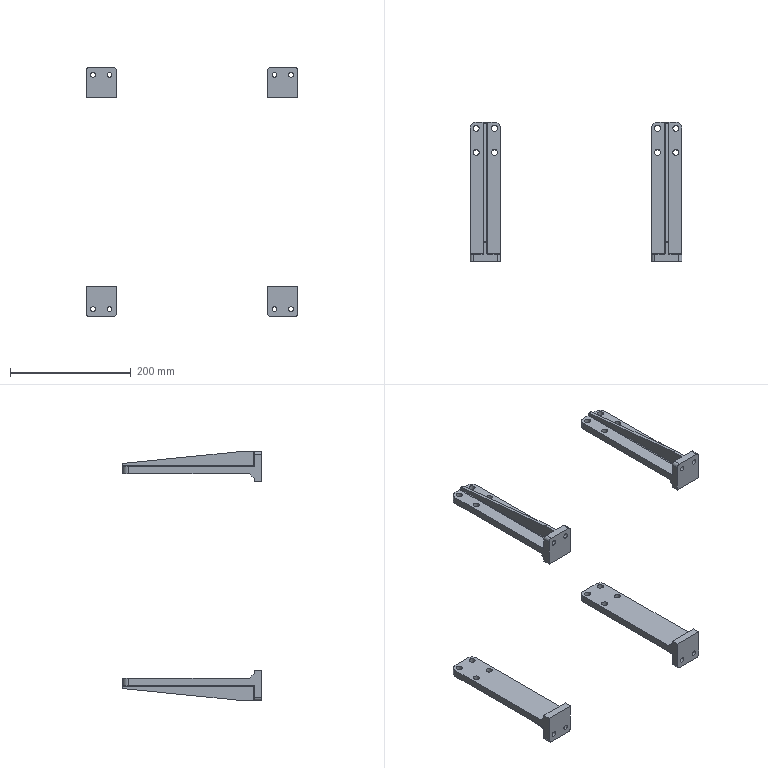Part | STEP file | Frame Combustor_1 | 4 solids | 144 faces | box 350 x 230 x 412 mm | volume 696961 mm3 | cylinder 72 | plane 64 | sphere 8 | commonest cylinder face diameters 2 x24 10 x24 4 x8 8 x8 20 x8